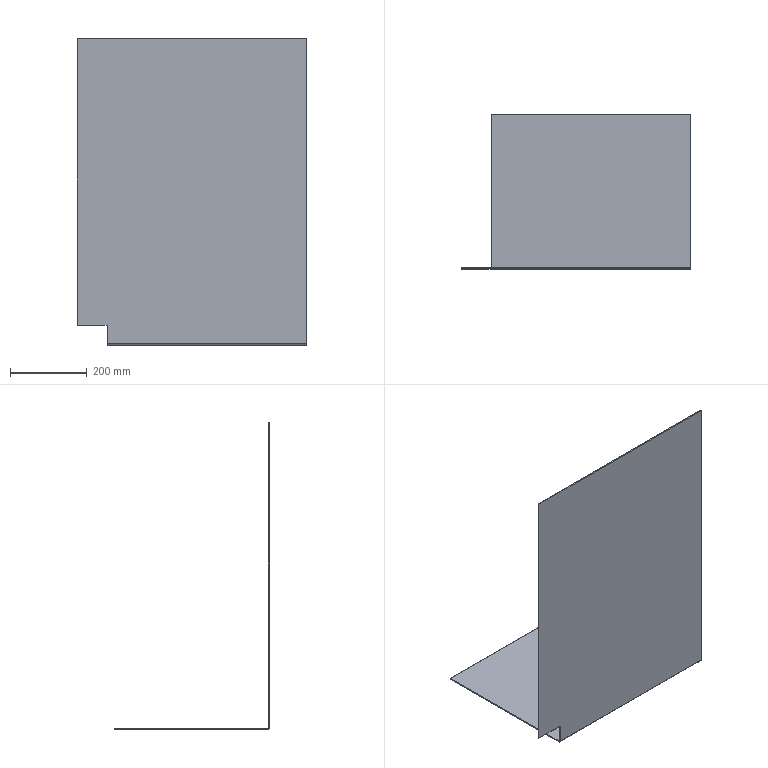Part | STEP file | E3-花纹Plate折弯5 | 1 solid | 14 faces | box 598 x 403 x 798 mm | volume 2041770 mm3 | plane 12 | cylinder 2 | commonest cylinder face diameters 2 x1 8 x1
STEP:
#1=CARTESIAN_POINT('',(0.,0.,0.));
#2=DIRECTION('',(0.,0.,1.));
#3=DIRECTION('',(1.,0.,0.));
#4=AXIS2_PLACEMENT_3D('',#1,#2,#3);
#5=CARTESIAN_POINT('',(598.,3.,-794.));
#6=VERTEX_POINT('',#5);
#7=CARTESIAN_POINT('',(598.,3.,0.));
#8=VERTEX_POINT('',#7);
#9=CARTESIAN_POINT('',(598.,3.,0.));
#10=DIRECTION('',(0.,0.,1.));
#11=VECTOR('',#10,1.);
#12=LINE('',#9,#11);
#13=CARTESIAN_POINT('',(598.,3.,0.));
#14=DIRECTION('',(1.,0.,0.));
#15=DIRECTION('',(0.,0.,1.));
#16=AXIS2_PLACEMENT_3D('',#13,#14,#15);
#17=PLANE('',#16);
#18=CARTESIAN_POINT('',(0.,0.));
#19=DIRECTION('',(1.,0.));
#20=VECTOR('',#19,1.);
#21=LINE('',#18,#20);
#22=(GEOMETRIC_REPRESENTATION_CONTEXT(2)PARAMETRIC_REPRESENTATION_CONTEXT()REPRESENTATION_CONTEXT('',''));
#23=DEFINITIONAL_REPRESENTATION('',(#21),#22);
#24=PCURVE('',#17,#23);
#25=CARTESIAN_POINT('',(0.,3.,0.));
#26=DIRECTION('',(0.,1.,0.));
#27=DIRECTION('',(0.,0.,-1.));
#28=AXIS2_PLACEMENT_3D('',#25,#26,#27);
#29=PLANE('',#28);
#30=CARTESIAN_POINT('',(0.,-598.));
#31=DIRECTION('',(-1.,0.));
#32=VECTOR('',#31,1.);
#33=LINE('',#30,#32);
#34=(GEOMETRIC_REPRESENTATION_CONTEXT(2)PARAMETRIC_REPRESENTATION_CONTEXT()REPRESENTATION_CONTEXT('',''));
#35=DEFINITIONAL_REPRESENTATION('',(#33),#34);
#36=PCURVE('',#29,#35);
#37=SURFACE_CURVE('',#12,(#24,#36),.PCURVE_S1.);
#38=EDGE_CURVE('',#6,#8,#37,.T.);
#39=ORIENTED_EDGE('',*,*,#38,.T.);
#40=CARTESIAN_POINT('',(598.,0.,0.));
#41=VERTEX_POINT('',#40);
#42=CARTESIAN_POINT('',(598.,3.,0.));
#43=DIRECTION('',(0.,1.,0.));
#44=VECTOR('',#43,1.);
#45=LINE('',#42,#44);
#46=CARTESIAN_POINT('',(0.,0.));
#47=DIRECTION('',(0.,-1.));
#48=VECTOR('',#47,1.);
#49=LINE('',#46,#48);
#50=(GEOMETRIC_REPRESENTATION_CONTEXT(2)PARAMETRIC_REPRESENTATION_CONTEXT()REPRESENTATION_CONTEXT('',''));
#51=DEFINITIONAL_REPRESENTATION('',(#49),#50);
#52=PCURVE('',#17,#51);
#53=CARTESIAN_POINT('',(0.,3.,0.));
#54=DIRECTION('',(0.,0.,1.));
#55=DIRECTION('',(-1.,0.,0.));
#56=AXIS2_PLACEMENT_3D('',#53,#54,#55);
#57=PLANE('',#56);
#58=CARTESIAN_POINT('',(-598.,0.));
#59=DIRECTION('',(0.,-1.));
#60=VECTOR('',#59,1.);
#61=LINE('',#58,#60);
#62=(GEOMETRIC_REPRESENTATION_CONTEXT(2)PARAMETRIC_REPRESENTATION_CONTEXT()REPRESENTATION_CONTEXT('',''));
#63=DEFINITIONAL_REPRESENTATION('',(#61),#62);
#64=PCURVE('',#57,#63);
#65=SURFACE_CURVE('',#45,(#52,#64),.PCURVE_S1.);
#66=EDGE_CURVE('',#41,#8,#65,.T.);
#67=ORIENTED_EDGE('',*,*,#66,.F.);
#68=CARTESIAN_POINT('',(598.,0.,-794.));
#69=VERTEX_POINT('',#68);
#70=CARTESIAN_POINT('',(598.,0.,0.));
#71=DIRECTION('',(0.,0.,1.));
#72=VECTOR('',#71,1.);
#73=LINE('',#70,#72);
#74=CARTESIAN_POINT('',(0.,3.));
#75=DIRECTION('',(1.,0.));
#76=VECTOR('',#75,1.);
#77=LINE('',#74,#76);
#78=(GEOMETRIC_REPRESENTATION_CONTEXT(2)PARAMETRIC_REPRESENTATION_CONTEXT()REPRESENTATION_CONTEXT('',''));
#79=DEFINITIONAL_REPRESENTATION('',(#77),#78);
#80=PCURVE('',#17,#79);
#81=CARTESIAN_POINT('',(0.,0.,0.));
#82=DIRECTION('',(0.,1.,0.));
#83=DIRECTION('',(0.,0.,-1.));
#84=AXIS2_PLACEMENT_3D('',#81,#82,#83);
#85=PLANE('',#84);
#86=CARTESIAN_POINT('',(0.,-598.));
#87=DIRECTION('',(-1.,0.));
#88=VECTOR('',#87,1.);
#89=LINE('',#86,#88);
#90=(GEOMETRIC_REPRESENTATION_CONTEXT(2)PARAMETRIC_REPRESENTATION_CONTEXT()REPRESENTATION_CONTEXT('',''));
#91=DEFINITIONAL_REPRESENTATION('',(#89),#90);
#92=PCURVE('',#85,#91);
#93=SURFACE_CURVE('',#73,(#80,#92),.PCURVE_S1.);
#94=EDGE_CURVE('',#69,#41,#93,.T.);
#95=ORIENTED_EDGE('',*,*,#94,.F.);
#96=CARTESIAN_POINT('',(598.,3.,-794.));
#97=DIRECTION('',(0.,-1.,0.));
#98=VECTOR('',#97,1.);
#99=LINE('',#96,#98);
#100=CARTESIAN_POINT('',(-794.,0.));
#101=DIRECTION('',(0.,1.));
#102=VECTOR('',#101,1.);
#103=LINE('',#100,#102);
#104=(GEOMETRIC_REPRESENTATION_CONTEXT(2)PARAMETRIC_REPRESENTATION_CONTEXT()REPRESENTATION_CONTEXT('',''));
#105=DEFINITIONAL_REPRESENTATION('',(#103),#104);
#106=PCURVE('',#17,#105);
#107=CARTESIAN_POINT('',(598.,4.,-794.));
#108=DIRECTION('',(-1.,0.,0.));
#109=DIRECTION('',(0.,0.,-1.));
#110=AXIS2_PLACEMENT_3D('',#107,#108,#109);
#111=PLANE('',#110);
#112=CARTESIAN_POINT('',(0.,1.));
#113=DIRECTION('',(0.,1.));
#114=VECTOR('',#113,1.);
#115=LINE('',#112,#114);
#116=(GEOMETRIC_REPRESENTATION_CONTEXT(2)PARAMETRIC_REPRESENTATION_CONTEXT()REPRESENTATION_CONTEXT('',''));
#117=DEFINITIONAL_REPRESENTATION('',(#115),#116);
#118=PCURVE('',#111,#117);
#119=SURFACE_CURVE('',#99,(#106,#118),.PCURVE_S1.);
#120=EDGE_CURVE('',#6,#69,#119,.T.);
#121=ORIENTED_EDGE('',*,*,#120,.F.);
#122=EDGE_LOOP('',(#39,#67,#95,#121));
#123=FACE_BOUND('',#122,.T.);
#124=ADVANCED_FACE('',(#123),#17,.T.);
#125=CARTESIAN_POINT('',(78.,3.,-746.));
#126=VERTEX_POINT('',#125);
#127=CARTESIAN_POINT('',(0.,3.,-746.));
#128=VERTEX_POINT('',#127);
#129=CARTESIAN_POINT('',(0.,3.,-746.));
#130=DIRECTION('',(-1.,0.,0.));
#131=VECTOR('',#130,1.);
#132=LINE('',#129,#131);
#133=CARTESIAN_POINT('',(746.,0.));
#134=DIRECTION('',(0.,1.));
#135=VECTOR('',#134,1.);
#136=LINE('',#133,#135);
#137=(GEOMETRIC_REPRESENTATION_CONTEXT(2)PARAMETRIC_REPRESENTATION_CONTEXT()REPRESENTATION_CONTEXT('',''));
#138=DEFINITIONAL_REPRESENTATION('',(#136),#137);
#139=PCURVE('',#29,#138);
#140=CARTESIAN_POINT('',(-82.,-497.,-746.));
#141=DIRECTION('',(0.,0.,1.));
#142=DIRECTION('',(-1.,0.,0.));
#143=AXIS2_PLACEMENT_3D('',#140,#141,#142);
#144=PLANE('',#143);
#145=CARTESIAN_POINT('',(-82.,-500.));
#146=DIRECTION('',(1.,0.));
#147=VECTOR('',#146,1.);
#148=LINE('',#145,#147);
#149=(GEOMETRIC_REPRESENTATION_CONTEXT(2)PARAMETRIC_REPRESENTATION_CONTEXT()REPRESENTATION_CONTEXT('',''));
#150=DEFINITIONAL_REPRESENTATION('',(#148),#149);
#151=PCURVE('',#144,#150);
#152=SURFACE_CURVE('',#132,(#139,#151),.PCURVE_S1.);
#153=EDGE_CURVE('',#126,#128,#152,.T.);
#154=ORIENTED_EDGE('',*,*,#153,.T.);
#155=CARTESIAN_POINT('',(0.,3.,0.));
#156=VERTEX_POINT('',#155);
#157=CARTESIAN_POINT('',(0.,3.,0.));
#158=DIRECTION('',(0.,0.,-1.));
#159=VECTOR('',#158,1.);
#160=LINE('',#157,#159);
#161=CARTESIAN_POINT('',(0.,0.));
#162=DIRECTION('',(1.,0.));
#163=VECTOR('',#162,1.);
#164=LINE('',#161,#163);
#165=(GEOMETRIC_REPRESENTATION_CONTEXT(2)PARAMETRIC_REPRESENTATION_CONTEXT()REPRESENTATION_CONTEXT('',''));
#166=DEFINITIONAL_REPRESENTATION('',(#164),#165);
#167=PCURVE('',#29,#166);
#168=CARTESIAN_POINT('',(0.,3.,0.));
#169=DIRECTION('',(-1.,0.,0.));
#170=DIRECTION('',(0.,0.,-1.));
#171=AXIS2_PLACEMENT_3D('',#168,#169,#170);
#172=PLANE('',#171);
#173=CARTESIAN_POINT('',(0.,0.));
#174=DIRECTION('',(1.,0.));
#175=VECTOR('',#174,1.);
#176=LINE('',#173,#175);
#177=(GEOMETRIC_REPRESENTATION_CONTEXT(2)PARAMETRIC_REPRESENTATION_CONTEXT()REPRESENTATION_CONTEXT('',''));
#178=DEFINITIONAL_REPRESENTATION('',(#176),#177);
#179=PCURVE('',#172,#178);
#180=SURFACE_CURVE('',#160,(#167,#179),.PCURVE_S1.);
#181=EDGE_CURVE('',#156,#128,#180,.T.);
#182=ORIENTED_EDGE('',*,*,#181,.F.);
#183=CARTESIAN_POINT('',(0.,3.,0.));
#184=DIRECTION('',(-1.,0.,0.));
#185=VECTOR('',#184,1.);
#186=LINE('',#183,#185);
#187=CARTESIAN_POINT('',(0.,0.));
#188=DIRECTION('',(0.,1.));
#189=VECTOR('',#188,1.);
#190=LINE('',#187,#189);
#191=(GEOMETRIC_REPRESENTATION_CONTEXT(2)PARAMETRIC_REPRESENTATION_CONTEXT()REPRESENTATION_CONTEXT('',''));
#192=DEFINITIONAL_REPRESENTATION('',(#190),#191);
#193=PCURVE('',#29,#192);
#194=CARTESIAN_POINT('',(0.,0.));
#195=DIRECTION('',(1.,0.));
#196=VECTOR('',#195,1.);
#197=LINE('',#194,#196);
#198=(GEOMETRIC_REPRESENTATION_CONTEXT(2)PARAMETRIC_REPRESENTATION_CONTEXT()REPRESENTATION_CONTEXT('',''));
#199=DEFINITIONAL_REPRESENTATION('',(#197),#198);
#200=PCURVE('',#57,#199);
#201=SURFACE_CURVE('',#186,(#193,#200),.PCURVE_S1.);
#202=EDGE_CURVE('',#8,#156,#201,.T.);
#203=ORIENTED_EDGE('',*,*,#202,.F.);
#204=ORIENTED_EDGE('',*,*,#38,.F.);
#205=CARTESIAN_POINT('',(78.,3.,-794.));
#206=VERTEX_POINT('',#205);
#207=CARTESIAN_POINT('',(598.,3.,-794.));
#208=DIRECTION('',(-1.,0.,0.));
#209=VECTOR('',#208,1.);
#210=LINE('',#207,#209);
#211=CARTESIAN_POINT('',(794.,-598.));
#212=DIRECTION('',(0.,1.));
#213=VECTOR('',#212,1.);
#214=LINE('',#211,#213);
#215=(GEOMETRIC_REPRESENTATION_CONTEXT(2)PARAMETRIC_REPRESENTATION_CONTEXT()REPRESENTATION_CONTEXT('',''));
#216=DEFINITIONAL_REPRESENTATION('',(#214),#215);
#217=PCURVE('',#29,#216);
#218=CARTESIAN_POINT('',(598.,4.,-794.));
#219=DIRECTION('',(1.,0.,0.));
#220=DIRECTION('',(0.,0.,-1.));
#221=AXIS2_PLACEMENT_3D('',#218,#219,#220);
#222=CYLINDRICAL_SURFACE('',#221,1.);
#223=CARTESIAN_POINT('',(4.712,0.));
#224=DIRECTION('',(0.,-1.));
#225=VECTOR('',#224,1.);
#226=LINE('',#223,#225);
#227=(GEOMETRIC_REPRESENTATION_CONTEXT(2)PARAMETRIC_REPRESENTATION_CONTEXT()REPRESENTATION_CONTEXT('',''));
#228=DEFINITIONAL_REPRESENTATION('',(#226),#227);
#229=PCURVE('',#222,#228);
#230=SURFACE_CURVE('',#210,(#217,#229),.PCURVE_S1.);
#231=EDGE_CURVE('',#6,#206,#230,.T.);
#232=ORIENTED_EDGE('',*,*,#231,.T.);
#233=CARTESIAN_POINT('',(78.,3.,0.));
#234=DIRECTION('',(0.,0.,1.));
#235=VECTOR('',#234,1.);
#236=LINE('',#233,#235);
#237=CARTESIAN_POINT('',(0.,-78.));
#238=DIRECTION('',(-1.,0.));
#239=VECTOR('',#238,1.);
#240=LINE('',#237,#239);
#241=(GEOMETRIC_REPRESENTATION_CONTEXT(2)PARAMETRIC_REPRESENTATION_CONTEXT()REPRESENTATION_CONTEXT('',''));
#242=DEFINITIONAL_REPRESENTATION('',(#240),#241);
#243=PCURVE('',#29,#242);
#244=CARTESIAN_POINT('',(78.,-497.,-798.));
#245=DIRECTION('',(1.,0.,0.));
#246=DIRECTION('',(0.,0.,1.));
#247=AXIS2_PLACEMENT_3D('',#244,#245,#246);
#248=PLANE('',#247);
#249=CARTESIAN_POINT('',(798.,-500.));
#250=DIRECTION('',(1.,0.));
#251=VECTOR('',#250,1.);
#252=LINE('',#249,#251);
#253=(GEOMETRIC_REPRESENTATION_CONTEXT(2)PARAMETRIC_REPRESENTATION_CONTEXT()REPRESENTATION_CONTEXT('',''));
#254=DEFINITIONAL_REPRESENTATION('',(#252),#253);
#255=PCURVE('',#248,#254);
#256=SURFACE_CURVE('',#236,(#243,#255),.PCURVE_S1.);
#257=EDGE_CURVE('',#206,#126,#256,.T.);
#258=ORIENTED_EDGE('',*,*,#257,.T.);
#259=EDGE_LOOP('',(#154,#182,#203,#204,#232,#258));
#260=FACE_BOUND('',#259,.T.);
#261=ADVANCED_FACE('',(#260),#29,.T.);
#262=CARTESIAN_POINT('',(78.,0.,-794.));
#263=VERTEX_POINT('',#262);
#264=CARTESIAN_POINT('',(78.,0.,-746.));
#265=VERTEX_POINT('',#264);
#266=CARTESIAN_POINT('',(78.,0.,0.));
#267=DIRECTION('',(0.,0.,1.));
#268=VECTOR('',#267,1.);
#269=LINE('',#266,#268);
#270=CARTESIAN_POINT('',(0.,-78.));
#271=DIRECTION('',(-1.,0.));
#272=VECTOR('',#271,1.);
#273=LINE('',#270,#272);
#274=(GEOMETRIC_REPRESENTATION_CONTEXT(2)PARAMETRIC_REPRESENTATION_CONTEXT()REPRESENTATION_CONTEXT('',''));
#275=DEFINITIONAL_REPRESENTATION('',(#273),#274);
#276=PCURVE('',#85,#275);
#277=CARTESIAN_POINT('',(798.,-497.));
#278=DIRECTION('',(1.,0.));
#279=VECTOR('',#278,1.);
#280=LINE('',#277,#279);
#281=(GEOMETRIC_REPRESENTATION_CONTEXT(2)PARAMETRIC_REPRESENTATION_CONTEXT()REPRESENTATION_CONTEXT('',''));
#282=DEFINITIONAL_REPRESENTATION('',(#280),#281);
#283=PCURVE('',#248,#282);
#284=SURFACE_CURVE('',#269,(#276,#283),.PCURVE_S1.);
#285=EDGE_CURVE('',#263,#265,#284,.T.);
#286=ORIENTED_EDGE('',*,*,#285,.F.);
#287=CARTESIAN_POINT('',(598.,0.,-794.));
#288=DIRECTION('',(-1.,0.,0.));
#289=VECTOR('',#288,1.);
#290=LINE('',#287,#289);
#291=CARTESIAN_POINT('',(794.,-598.));
#292=DIRECTION('',(0.,1.));
#293=VECTOR('',#292,1.);
#294=LINE('',#291,#293);
#295=(GEOMETRIC_REPRESENTATION_CONTEXT(2)PARAMETRIC_REPRESENTATION_CONTEXT()REPRESENTATION_CONTEXT('',''));
#296=DEFINITIONAL_REPRESENTATION('',(#294),#295);
#297=PCURVE('',#85,#296);
#298=CARTESIAN_POINT('',(598.,4.,-794.));
#299=DIRECTION('',(1.,0.,0.));
#300=DIRECTION('',(0.,0.,-1.));
#301=AXIS2_PLACEMENT_3D('',#298,#299,#300);
#302=CYLINDRICAL_SURFACE('',#301,4.);
#303=CARTESIAN_POINT('',(4.712,0.));
#304=DIRECTION('',(0.,-1.));
#305=VECTOR('',#304,1.);
#306=LINE('',#303,#305);
#307=(GEOMETRIC_REPRESENTATION_CONTEXT(2)PARAMETRIC_REPRESENTATION_CONTEXT()REPRESENTATION_CONTEXT('',''));
#308=DEFINITIONAL_REPRESENTATION('',(#306),#307);
#309=PCURVE('',#302,#308);
#310=SURFACE_CURVE('',#290,(#297,#309),.PCURVE_S1.);
#311=EDGE_CURVE('',#69,#263,#310,.T.);
#312=ORIENTED_EDGE('',*,*,#311,.F.);
#313=ORIENTED_EDGE('',*,*,#94,.T.);
#314=CARTESIAN_POINT('',(0.,0.,0.));
#315=VERTEX_POINT('',#314);
#316=CARTESIAN_POINT('',(0.,0.,0.));
#317=DIRECTION('',(-1.,0.,0.));
#318=VECTOR('',#317,1.);
#319=LINE('',#316,#318);
#320=CARTESIAN_POINT('',(0.,0.));
#321=DIRECTION('',(0.,1.));
#322=VECTOR('',#321,1.);
#323=LINE('',#320,#322);
#324=(GEOMETRIC_REPRESENTATION_CONTEXT(2)PARAMETRIC_REPRESENTATION_CONTEXT()REPRESENTATION_CONTEXT('',''));
#325=DEFINITIONAL_REPRESENTATION('',(#323),#324);
#326=PCURVE('',#85,#325);
#327=CARTESIAN_POINT('',(0.,3.));
#328=DIRECTION('',(1.,0.));
#329=VECTOR('',#328,1.);
#330=LINE('',#327,#329);
#331=(GEOMETRIC_REPRESENTATION_CONTEXT(2)PARAMETRIC_REPRESENTATION_CONTEXT()REPRESENTATION_CONTEXT('',''));
#332=DEFINITIONAL_REPRESENTATION('',(#330),#331);
#333=PCURVE('',#57,#332);
#334=SURFACE_CURVE('',#319,(#326,#333),.PCURVE_S1.);
#335=EDGE_CURVE('',#41,#315,#334,.T.);
#336=ORIENTED_EDGE('',*,*,#335,.T.);
#337=CARTESIAN_POINT('',(0.,0.,-746.));
#338=VERTEX_POINT('',#337);
#339=CARTESIAN_POINT('',(0.,0.,0.));
#340=DIRECTION('',(0.,0.,-1.));
#341=VECTOR('',#340,1.);
#342=LINE('',#339,#341);
#343=CARTESIAN_POINT('',(0.,0.));
#344=DIRECTION('',(1.,0.));
#345=VECTOR('',#344,1.);
#346=LINE('',#343,#345);
#347=(GEOMETRIC_REPRESENTATION_CONTEXT(2)PARAMETRIC_REPRESENTATION_CONTEXT()REPRESENTATION_CONTEXT('',''));
#348=DEFINITIONAL_REPRESENTATION('',(#346),#347);
#349=PCURVE('',#85,#348);
#350=CARTESIAN_POINT('',(0.,3.));
#351=DIRECTION('',(1.,0.));
#352=VECTOR('',#351,1.);
#353=LINE('',#350,#352);
#354=(GEOMETRIC_REPRESENTATION_CONTEXT(2)PARAMETRIC_REPRESENTATION_CONTEXT()REPRESENTATION_CONTEXT('',''));
#355=DEFINITIONAL_REPRESENTATION('',(#353),#354);
#356=PCURVE('',#172,#355);
#357=SURFACE_CURVE('',#342,(#349,#356),.PCURVE_S1.);
#358=EDGE_CURVE('',#315,#338,#357,.T.);
#359=ORIENTED_EDGE('',*,*,#358,.T.);
#360=CARTESIAN_POINT('',(0.,0.,-746.));
#361=DIRECTION('',(-1.,0.,0.));
#362=VECTOR('',#361,1.);
#363=LINE('',#360,#362);
#364=CARTESIAN_POINT('',(746.,0.));
#365=DIRECTION('',(0.,1.));
#366=VECTOR('',#365,1.);
#367=LINE('',#364,#366);
#368=(GEOMETRIC_REPRESENTATION_CONTEXT(2)PARAMETRIC_REPRESENTATION_CONTEXT()REPRESENTATION_CONTEXT('',''));
#369=DEFINITIONAL_REPRESENTATION('',(#367),#368);
#370=PCURVE('',#85,#369);
#371=CARTESIAN_POINT('',(-82.,-497.));
#372=DIRECTION('',(1.,0.));
#373=VECTOR('',#372,1.);
#374=LINE('',#371,#373);
#375=(GEOMETRIC_REPRESENTATION_CONTEXT(2)PARAMETRIC_REPRESENTATION_CONTEXT()REPRESENTATION_CONTEXT('',''));
#376=DEFINITIONAL_REPRESENTATION('',(#374),#375);
#377=PCURVE('',#144,#376);
#378=SURFACE_CURVE('',#363,(#370,#377),.PCURVE_S1.);
#379=EDGE_CURVE('',#265,#338,#378,.T.);
#380=ORIENTED_EDGE('',*,*,#379,.F.);
#381=EDGE_LOOP('',(#286,#312,#313,#336,#359,#380));
#382=FACE_BOUND('',#381,.T.);
#383=ADVANCED_FACE('',(#382),#85,.F.);
#384=ORIENTED_EDGE('',*,*,#66,.T.);
#385=ORIENTED_EDGE('',*,*,#202,.T.);
#386=CARTESIAN_POINT('',(0.,3.,0.));
#387=DIRECTION('',(0.,1.,0.));
#388=VECTOR('',#387,1.);
#389=LINE('',#386,#388);
#390=CARTESIAN_POINT('',(0.,0.));
#391=DIRECTION('',(0.,-1.));
#392=VECTOR('',#391,1.);
#393=LINE('',#390,#392);
#394=(GEOMETRIC_REPRESENTATION_CONTEXT(2)PARAMETRIC_REPRESENTATION_CONTEXT()REPRESENTATION_CONTEXT('',''));
#395=DEFINITIONAL_REPRESENTATION('',(#393),#394);
#396=PCURVE('',#57,#395);
#397=CARTESIAN_POINT('',(0.,0.));
#398=DIRECTION('',(0.,-1.));
#399=VECTOR('',#398,1.);
#400=LINE('',#397,#399);
#401=(GEOMETRIC_REPRESENTATION_CONTEXT(2)PARAMETRIC_REPRESENTATION_CONTEXT()REPRESENTATION_CONTEXT('',''));
#402=DEFINITIONAL_REPRESENTATION('',(#400),#401);
#403=PCURVE('',#172,#402);
#404=SURFACE_CURVE('',#389,(#396,#403),.PCURVE_S1.);
#405=EDGE_CURVE('',#315,#156,#404,.T.);
#406=ORIENTED_EDGE('',*,*,#405,.F.);
#407=ORIENTED_EDGE('',*,*,#335,.F.);
#408=EDGE_LOOP('',(#384,#385,#406,#407));
#409=FACE_BOUND('',#408,.T.);
#410=ADVANCED_FACE('',(#409),#57,.T.);
#411=CARTESIAN_POINT('',(0.,3.,-746.));
#412=DIRECTION('',(0.,-1.,0.));
#413=VECTOR('',#412,1.);
#414=LINE('',#411,#413);
#415=CARTESIAN_POINT('',(746.,0.));
#416=DIRECTION('',(0.,1.));
#417=VECTOR('',#416,1.);
#418=LINE('',#415,#417);
#419=(GEOMETRIC_REPRESENTATION_CONTEXT(2)PARAMETRIC_REPRESENTATION_CONTEXT()REPRESENTATION_CONTEXT('',''));
#420=DEFINITIONAL_REPRESENTATION('',(#418),#419);
#421=PCURVE('',#172,#420);
#422=CARTESIAN_POINT('',(-82.,-500.));
#423=DIRECTION('',(0.,1.));
#424=VECTOR('',#423,1.);
#425=LINE('',#422,#424);
#426=(GEOMETRIC_REPRESENTATION_CONTEXT(2)PARAMETRIC_REPRESENTATION_CONTEXT()REPRESENTATION_CONTEXT('',''));
#427=DEFINITIONAL_REPRESENTATION('',(#425),#426);
#428=PCURVE('',#144,#427);
#429=SURFACE_CURVE('',#414,(#421,#428),.PCURVE_S1.);
#430=EDGE_CURVE('',#128,#338,#429,.T.);
#431=ORIENTED_EDGE('',*,*,#430,.T.);
#432=ORIENTED_EDGE('',*,*,#358,.F.);
#433=ORIENTED_EDGE('',*,*,#405,.T.);
#434=ORIENTED_EDGE('',*,*,#181,.T.);
#435=EDGE_LOOP('',(#431,#432,#433,#434));
#436=FACE_BOUND('',#435,.T.);
#437=ADVANCED_FACE('',(#436),#172,.T.);
#438=CARTESIAN_POINT('',(598.,4.,-795.));
#439=VERTEX_POINT('',#438);
#440=CARTESIAN_POINT('',(598.,4.,-794.));
#441=DIRECTION('',(-1.,0.,0.));
#442=DIRECTION('',(0.,0.,1.));
#443=AXIS2_PLACEMENT_3D('',#440,#441,#442);
#444=CIRCLE('',#443,1.);
#445=CARTESIAN_POINT('',(0.,0.));
#446=DIRECTION('',(-1.,0.));
#447=AXIS2_PLACEMENT_2D('',#445,#446);
#448=CIRCLE('',#447,1.);
#449=(GEOMETRIC_REPRESENTATION_CONTEXT(2)PARAMETRIC_REPRESENTATION_CONTEXT()REPRESENTATION_CONTEXT('',''));
#450=DEFINITIONAL_REPRESENTATION('',(#448),#449);
#451=PCURVE('',#111,#450);
#452=CARTESIAN_POINT('',(9.425,0.));
#453=DIRECTION('',(-1.,0.));
#454=VECTOR('',#453,1.);
#455=LINE('',#452,#454);
#456=(GEOMETRIC_REPRESENTATION_CONTEXT(2)PARAMETRIC_REPRESENTATION_CONTEXT()REPRESENTATION_CONTEXT('',''));
#457=DEFINITIONAL_REPRESENTATION('',(#455),#456);
#458=PCURVE('',#222,#457);
#459=SURFACE_CURVE('',#444,(#451,#458),.PCURVE_S1.);
#460=EDGE_CURVE('',#439,#6,#459,.T.);
#461=ORIENTED_EDGE('',*,*,#460,.T.);
#462=ORIENTED_EDGE('',*,*,#120,.T.);
#463=CARTESIAN_POINT('',(598.,4.,-798.));
#464=VERTEX_POINT('',#463);
#465=CARTESIAN_POINT('',(598.,4.,-794.));
#466=DIRECTION('',(-1.,0.,0.));
#467=DIRECTION('',(0.,0.,1.));
#468=AXIS2_PLACEMENT_3D('',#465,#466,#467);
#469=CIRCLE('',#468,4.);
#470=CARTESIAN_POINT('',(0.,0.));
#471=DIRECTION('',(-1.,0.));
#472=AXIS2_PLACEMENT_2D('',#470,#471);
#473=CIRCLE('',#472,4.);
#474=(GEOMETRIC_REPRESENTATION_CONTEXT(2)PARAMETRIC_REPRESENTATION_CONTEXT()REPRESENTATION_CONTEXT('',''));
#475=DEFINITIONAL_REPRESENTATION('',(#473),#474);
#476=PCURVE('',#111,#475);
#477=CARTESIAN_POINT('',(9.425,0.));
#478=DIRECTION('',(-1.,0.));
#479=VECTOR('',#478,1.);
#480=LINE('',#477,#479);
#481=(GEOMETRIC_REPRESENTATION_CONTEXT(2)PARAMETRIC_REPRESENTATION_CONTEXT()REPRESENTATION_CONTEXT('',''));
#482=DEFINITIONAL_REPRESENTATION('',(#480),#481);
#483=PCURVE('',#302,#482);
#484=SURFACE_CURVE('',#469,(#476,#483),.PCURVE_S1.);
#485=EDGE_CURVE('',#464,#69,#484,.T.);
#486=ORIENTED_EDGE('',*,*,#485,.F.);
#487=CARTESIAN_POINT('',(598.,4.,-795.));
#488=DIRECTION('',(0.,0.,-1.));
#489=VECTOR('',#488,1.);
#490=LINE('',#487,#489);
#491=CARTESIAN_POINT('',(1.,0.));
#492=DIRECTION('',(1.,0.));
#493=VECTOR('',#492,1.);
#494=LINE('',#491,#493);
#495=(GEOMETRIC_REPRESENTATION_CONTEXT(2)PARAMETRIC_REPRESENTATION_CONTEXT()REPRESENTATION_CONTEXT('',''));
#496=DEFINITIONAL_REPRESENTATION('',(#494),#495);
#497=PCURVE('',#111,#496);
#498=CARTESIAN_POINT('',(598.,403.,-798.));
#499=DIRECTION('',(-1.,0.,0.));
#500=DIRECTION('',(0.,0.,-1.));
#501=AXIS2_PLACEMENT_3D('',#498,#499,#500);
#502=PLANE('',#501);
#503=CARTESIAN_POINT('',(-3.,399.));
#504=DIRECTION('',(1.,0.));
#505=VECTOR('',#504,1.);
#506=LINE('',#503,#505);
#507=(GEOMETRIC_REPRESENTATION_CONTEXT(2)PARAMETRIC_REPRESENTATION_CONTEXT()REPRESENTATION_CONTEXT('',''));
#508=DEFINITIONAL_REPRESENTATION('',(#506),#507);
#509=PCURVE('',#502,#508);
#510=SURFACE_CURVE('',#490,(#497,#509),.PCURVE_S1.);
#511=EDGE_CURVE('',#439,#464,#510,.T.);
#512=ORIENTED_EDGE('',*,*,#511,.F.);
#513=EDGE_LOOP('',(#461,#462,#486,#512));
#514=FACE_BOUND('',#513,.T.);
#515=ADVANCED_FACE('',(#514),#111,.F.);
#516=CARTESIAN_POINT('',(78.,4.,-798.));
#517=VERTEX_POINT('',#516);
#518=CARTESIAN_POINT('',(78.,4.,-794.));
#519=DIRECTION('',(1.,0.,0.));
#520=DIRECTION('',(0.,0.,1.));
#521=AXIS2_PLACEMENT_3D('',#518,#519,#520);
#522=CIRCLE('',#521,4.);
#523=CARTESIAN_POINT('',(3.142,-520.));
#524=DIRECTION('',(1.,0.));
#525=VECTOR('',#524,1.);
#526=LINE('',#523,#525);
#527=(GEOMETRIC_REPRESENTATION_CONTEXT(2)PARAMETRIC_REPRESENTATION_CONTEXT()REPRESENTATION_CONTEXT('',''));
#528=DEFINITIONAL_REPRESENTATION('',(#526),#527);
#529=PCURVE('',#302,#528);
#530=CARTESIAN_POINT('',(4.,-501.));
#531=DIRECTION('',(1.,0.));
#532=AXIS2_PLACEMENT_2D('',#530,#531);
#533=CIRCLE('',#532,4.);
#534=(GEOMETRIC_REPRESENTATION_CONTEXT(2)PARAMETRIC_REPRESENTATION_CONTEXT()REPRESENTATION_CONTEXT('',''));
#535=DEFINITIONAL_REPRESENTATION('',(#533),#534);
#536=PCURVE('',#248,#535);
#537=SURFACE_CURVE('',#522,(#529,#536),.PCURVE_S1.);
#538=EDGE_CURVE('',#263,#517,#537,.T.);
#539=ORIENTED_EDGE('',*,*,#538,.T.);
#540=CARTESIAN_POINT('',(0.,4.,-798.));
#541=DIRECTION('',(-1.,0.,0.));
#542=VECTOR('',#541,1.);
#543=LINE('',#540,#542);
#544=CARTESIAN_POINT('',(6.283,-598.));
#545=DIRECTION('',(0.,-1.));
#546=VECTOR('',#545,1.);
#547=LINE('',#544,#546);
#548=(GEOMETRIC_REPRESENTATION_CONTEXT(2)PARAMETRIC_REPRESENTATION_CONTEXT()REPRESENTATION_CONTEXT('',''));
#549=DEFINITIONAL_REPRESENTATION('',(#547),#548);
#550=PCURVE('',#302,#549);
#551=CARTESIAN_POINT('',(0.,0.,-798.));
#552=DIRECTION('',(0.,0.,1.));
#553=DIRECTION('',(-1.,0.,0.));
#554=AXIS2_PLACEMENT_3D('',#551,#552,#553);
#555=PLANE('',#554);
#556=CARTESIAN_POINT('',(0.,-4.));
#557=DIRECTION('',(1.,0.));
#558=VECTOR('',#557,1.);
#559=LINE('',#556,#558);
#560=(GEOMETRIC_REPRESENTATION_CONTEXT(2)PARAMETRIC_REPRESENTATION_CONTEXT()REPRESENTATION_CONTEXT('',''));
#561=DEFINITIONAL_REPRESENTATION('',(#559),#560);
#562=PCURVE('',#555,#561);
#563=SURFACE_CURVE('',#543,(#550,#562),.PCURVE_S1.);
#564=EDGE_CURVE('',#464,#517,#563,.T.);
#565=ORIENTED_EDGE('',*,*,#564,.F.);
#566=ORIENTED_EDGE('',*,*,#485,.T.);
#567=ORIENTED_EDGE('',*,*,#311,.T.);
#568=EDGE_LOOP('',(#539,#565,#566,#567));
#569=FACE_BOUND('',#568,.T.);
#570=ADVANCED_FACE('',(#569),#302,.T.);
#571=CARTESIAN_POINT('',(78.,4.,-795.));
#572=VERTEX_POINT('',#571);
#573=CARTESIAN_POINT('',(78.,4.,-794.));
#574=DIRECTION('',(1.,0.,0.));
#575=DIRECTION('',(0.,0.,1.));
#576=AXIS2_PLACEMENT_3D('',#573,#574,#575);
#577=CIRCLE('',#576,1.);
#578=CARTESIAN_POINT('',(3.142,-520.));
#579=DIRECTION('',(1.,0.));
#580=VECTOR('',#579,1.);
#581=LINE('',#578,#580);
#582=(GEOMETRIC_REPRESENTATION_CONTEXT(2)PARAMETRIC_REPRESENTATION_CONTEXT()REPRESENTATION_CONTEXT('',''));
#583=DEFINITIONAL_REPRESENTATION('',(#581),#582);
#584=PCURVE('',#222,#583);
#585=CARTESIAN_POINT('',(4.,-501.));
#586=DIRECTION('',(1.,0.));
#587=AXIS2_PLACEMENT_2D('',#585,#586);
#588=CIRCLE('',#587,1.);
#589=(GEOMETRIC_REPRESENTATION_CONTEXT(2)PARAMETRIC_REPRESENTATION_CONTEXT()REPRESENTATION_CONTEXT('',''));
#590=DEFINITIONAL_REPRESENTATION('',(#588),#589);
#591=PCURVE('',#248,#590);
#592=SURFACE_CURVE('',#577,(#584,#591),.PCURVE_S1.);
#593=EDGE_CURVE('',#206,#572,#592,.T.);
#594=ORIENTED_EDGE('',*,*,#593,.T.);
#595=CARTESIAN_POINT('',(0.,4.,-795.));
#596=DIRECTION('',(1.,0.,0.));
#597=VECTOR('',#596,1.);
#598=LINE('',#595,#597);
#599=CARTESIAN_POINT('',(6.283,-598.));
#600=DIRECTION('',(0.,1.));
#601=VECTOR('',#600,1.);
#602=LINE('',#599,#601);
#603=(GEOMETRIC_REPRESENTATION_CONTEXT(2)PARAMETRIC_REPRESENTATION_CONTEXT()REPRESENTATION_CONTEXT('',''));
#604=DEFINITIONAL_REPRESENTATION('',(#602),#603);
#605=PCURVE('',#222,#604);
#606=CARTESIAN_POINT('',(0.,0.,-795.));
#607=DIRECTION('',(0.,0.,1.));
#608=DIRECTION('',(-1.,0.,0.));
#609=AXIS2_PLACEMENT_3D('',#606,#607,#608);
#610=PLANE('',#609);
#611=CARTESIAN_POINT('',(0.,-4.));
#612=DIRECTION('',(-1.,0.));
#613=VECTOR('',#612,1.);
#614=LINE('',#611,#613);
#615=(GEOMETRIC_REPRESENTATION_CONTEXT(2)PARAMETRIC_REPRESENTATION_CONTEXT()REPRESENTATION_CONTEXT('',''));
#616=DEFINITIONAL_REPRESENTATION('',(#614),#615);
#617=PCURVE('',#610,#616);
#618=SURFACE_CURVE('',#598,(#605,#617),.PCURVE_S1.);
#619=EDGE_CURVE('',#572,#439,#618,.T.);
#620=ORIENTED_EDGE('',*,*,#619,.T.);
#621=ORIENTED_EDGE('',*,*,#460,.T.);
#622=ORIENTED_EDGE('',*,*,#231,.T.);
#623=EDGE_LOOP('',(#594,#620,#621,#622));
#624=FACE_BOUND('',#623,.F.);
#625=ADVANCED_FACE('',(#624),#222,.F.);
#626=ORIENTED_EDGE('',*,*,#511,.T.);
#627=CARTESIAN_POINT('',(598.,403.,-798.));
#628=VERTEX_POINT('',#627);
#629=CARTESIAN_POINT('',(598.,0.,-798.));
#630=DIRECTION('',(0.,1.,0.));
#631=VECTOR('',#630,1.);
#632=LINE('',#629,#631);
#633=CARTESIAN_POINT('',(0.,403.));
#634=DIRECTION('',(0.,-1.));
#635=VECTOR('',#634,1.);
#636=LINE('',#633,#635);
#637=(GEOMETRIC_REPRESENTATION_CONTEXT(2)PARAMETRIC_REPRESENTATION_CONTEXT()REPRESENTATION_CONTEXT('',''));
#638=DEFINITIONAL_REPRESENTATION('',(#636),#637);
#639=PCURVE('',#502,#638);
#640=CARTESIAN_POINT('',(-598.,0.));
#641=DIRECTION('',(0.,-1.));
#642=VECTOR('',#641,1.);
#643=LINE('',#640,#642);
#644=(GEOMETRIC_REPRESENTATION_CONTEXT(2)PARAMETRIC_REPRESENTATION_CONTEXT()REPRESENTATION_CONTEXT('',''));
#645=DEFINITIONAL_REPRESENTATION('',(#643),#644);
#646=PCURVE('',#555,#645);
#647=SURFACE_CURVE('',#632,(#639,#646),.PCURVE_S1.);
#648=EDGE_CURVE('',#464,#628,#647,.T.);
#649=ORIENTED_EDGE('',*,*,#648,.T.);
#650=CARTESIAN_POINT('',(598.,403.,-795.));
#651=VERTEX_POINT('',#650);
#652=CARTESIAN_POINT('',(598.,403.,-798.));
#653=DIRECTION('',(0.,0.,1.));
#654=VECTOR('',#653,1.);
#655=LINE('',#652,#654);
#656=CARTESIAN_POINT('',(0.,0.));
#657=DIRECTION('',(-1.,0.));
#658=VECTOR('',#657,1.);
#659=LINE('',#656,#658);
#660=(GEOMETRIC_REPRESENTATION_CONTEXT(2)PARAMETRIC_REPRESENTATION_CONTEXT()REPRESENTATION_CONTEXT('',''));
#661=DEFINITIONAL_REPRESENTATION('',(#659),#660);
#662=PCURVE('',#502,#661);
#663=CARTESIAN_POINT('',(0.,403.,-798.));
#664=DIRECTION('',(0.,-1.,0.));
#665=DIRECTION('',(0.,0.,1.));
#666=AXIS2_PLACEMENT_3D('',#663,#664,#665);
#667=PLANE('',#666);
#668=CARTESIAN_POINT('',(0.,-598.));
#669=DIRECTION('',(1.,0.));
#670=VECTOR('',#669,1.);
#671=LINE('',#668,#670);
#672=(GEOMETRIC_REPRESENTATION_CONTEXT(2)PARAMETRIC_REPRESENTATION_CONTEXT()REPRESENTATION_CONTEXT('',''));
#673=DEFINITIONAL_REPRESENTATION('',(#671),#672);
#674=PCURVE('',#667,#673);
#675=SURFACE_CURVE('',#655,(#662,#674),.PCURVE_S1.);
#676=EDGE_CURVE('',#628,#651,#675,.T.);
#677=ORIENTED_EDGE('',*,*,#676,.T.);
#678=CARTESIAN_POINT('',(598.,403.,-795.));
#679=DIRECTION('',(0.,1.,0.));
#680=VECTOR('',#679,1.);
#681=LINE('',#678,#680);
#682=CARTESIAN_POINT('',(-3.,0.));
#683=DIRECTION('',(0.,-1.));
#684=VECTOR('',#683,1.);
#685=LINE('',#682,#684);
#686=(GEOMETRIC_REPRESENTATION_CONTEXT(2)PARAMETRIC_REPRESENTATION_CONTEXT()REPRESENTATION_CONTEXT('',''));
#687=DEFINITIONAL_REPRESENTATION('',(#685),#686);
#688=PCURVE('',#502,#687);
#689=CARTESIAN_POINT('',(-598.,-403.));
#690=DIRECTION('',(0.,-1.));
#691=VECTOR('',#690,1.);
#692=LINE('',#689,#691);
#693=(GEOMETRIC_REPRESENTATION_CONTEXT(2)PARAMETRIC_REPRESENTATION_CONTEXT()REPRESENTATION_CONTEXT('',''));
#694=DEFINITIONAL_REPRESENTATION('',(#692),#693);
#695=PCURVE('',#610,#694);
#696=SURFACE_CURVE('',#681,(#688,#695),.PCURVE_S1.);
#697=EDGE_CURVE('',#439,#651,#696,.T.);
#698=ORIENTED_EDGE('',*,*,#697,.F.);
#699=EDGE_LOOP('',(#626,#649,#677,#698));
#700=FACE_BOUND('',#699,.T.);
#701=ADVANCED_FACE('',(#700),#502,.F.);
#702=CARTESIAN_POINT('',(78.,403.,-798.));
#703=VERTEX_POINT('',#702);
#704=CARTESIAN_POINT('',(0.,403.,-798.));
#705=DIRECTION('',(-1.,0.,0.));
#706=VECTOR('',#705,1.);
#707=LINE('',#704,#706);
#708=CARTESIAN_POINT('',(0.,-403.));
#709=DIRECTION('',(1.,0.));
#710=VECTOR('',#709,1.);
#711=LINE('',#708,#710);
#712=(GEOMETRIC_REPRESENTATION_CONTEXT(2)PARAMETRIC_REPRESENTATION_CONTEXT()REPRESENTATION_CONTEXT('',''));
#713=DEFINITIONAL_REPRESENTATION('',(#711),#712);
#714=PCURVE('',#555,#713);
#715=CARTESIAN_POINT('',(0.,0.));
#716=DIRECTION('',(0.,1.));
#717=VECTOR('',#716,1.);
#718=LINE('',#715,#717);
#719=(GEOMETRIC_REPRESENTATION_CONTEXT(2)PARAMETRIC_REPRESENTATION_CONTEXT()REPRESENTATION_CONTEXT('',''));
#720=DEFINITIONAL_REPRESENTATION('',(#718),#719);
#721=PCURVE('',#667,#720);
#722=SURFACE_CURVE('',#707,(#714,#721),.PCURVE_S1.);
#723=EDGE_CURVE('',#628,#703,#722,.T.);
#724=ORIENTED_EDGE('',*,*,#723,.F.);
#725=ORIENTED_EDGE('',*,*,#648,.F.);
#726=ORIENTED_EDGE('',*,*,#564,.T.);
#727=CARTESIAN_POINT('',(78.,-497.,-798.));
#728=DIRECTION('',(0.,1.,0.));
#729=VECTOR('',#728,1.);
#730=LINE('',#727,#729);
#731=CARTESIAN_POINT('',(-78.,497.));
#732=DIRECTION('',(0.,-1.));
#733=VECTOR('',#732,1.);
#734=LINE('',#731,#733);
#735=(GEOMETRIC_REPRESENTATION_CONTEXT(2)PARAMETRIC_REPRESENTATION_CONTEXT()REPRESENTATION_CONTEXT('',''));
#736=DEFINITIONAL_REPRESENTATION('',(#734),#735);
#737=PCURVE('',#555,#736);
#738=CARTESIAN_POINT('',(0.,0.));
#739=DIRECTION('',(0.,-1.));
#740=VECTOR('',#739,1.);
#741=LINE('',#738,#740);
#742=(GEOMETRIC_REPRESENTATION_CONTEXT(2)PARAMETRIC_REPRESENTATION_CONTEXT()REPRESENTATION_CONTEXT('',''));
#743=DEFINITIONAL_REPRESENTATION('',(#741),#742);
#744=PCURVE('',#248,#743);
#745=SURFACE_CURVE('',#730,(#737,#744),.PCURVE_S1.);
#746=EDGE_CURVE('',#517,#703,#745,.T.);
#747=ORIENTED_EDGE('',*,*,#746,.T.);
#748=EDGE_LOOP('',(#724,#725,#726,#747));
#749=FACE_BOUND('',#748,.T.);
#750=ADVANCED_FACE('',(#749),#555,.F.);
#751=CARTESIAN_POINT('',(78.,403.,-795.));
#752=VERTEX_POINT('',#751);
#753=CARTESIAN_POINT('',(78.,0.,-795.));
#754=DIRECTION('',(0.,-1.,0.));
#755=VECTOR('',#754,1.);
#756=LINE('',#753,#755);
#757=CARTESIAN_POINT('',(-78.,0.));
#758=DIRECTION('',(0.,1.));
#759=VECTOR('',#758,1.);
#760=LINE('',#757,#759);
#761=(GEOMETRIC_REPRESENTATION_CONTEXT(2)PARAMETRIC_REPRESENTATION_CONTEXT()REPRESENTATION_CONTEXT('',''));
#762=DEFINITIONAL_REPRESENTATION('',(#760),#761);
#763=PCURVE('',#610,#762);
#764=CARTESIAN_POINT('',(3.,-497.));
#765=DIRECTION('',(0.,1.));
#766=VECTOR('',#765,1.);
#767=LINE('',#764,#766);
#768=(GEOMETRIC_REPRESENTATION_CONTEXT(2)PARAMETRIC_REPRESENTATION_CONTEXT()REPRESENTATION_CONTEXT('',''));
#769=DEFINITIONAL_REPRESENTATION('',(#767),#768);
#770=PCURVE('',#248,#769);
#771=SURFACE_CURVE('',#756,(#763,#770),.PCURVE_S1.);
#772=EDGE_CURVE('',#752,#572,#771,.T.);
#773=ORIENTED_EDGE('',*,*,#772,.T.);
#774=ORIENTED_EDGE('',*,*,#619,.T.);
#775=ORIENTED_EDGE('',*,*,#697,.T.);
#776=CARTESIAN_POINT('',(0.,403.,-795.));
#777=DIRECTION('',(-1.,0.,0.));
#778=VECTOR('',#777,1.);
#779=LINE('',#776,#778);
#780=CARTESIAN_POINT('',(0.,-403.));
#781=DIRECTION('',(1.,0.));
#782=VECTOR('',#781,1.);
#783=LINE('',#780,#782);
#784=(GEOMETRIC_REPRESENTATION_CONTEXT(2)PARAMETRIC_REPRESENTATION_CONTEXT()REPRESENTATION_CONTEXT('',''));
#785=DEFINITIONAL_REPRESENTATION('',(#783),#784);
#786=PCURVE('',#610,#785);
#787=CARTESIAN_POINT('',(3.,0.));
#788=DIRECTION('',(0.,1.));
#789=VECTOR('',#788,1.);
#790=LINE('',#787,#789);
#791=(GEOMETRIC_REPRESENTATION_CONTEXT(2)PARAMETRIC_REPRESENTATION_CONTEXT()REPRESENTATION_CONTEXT('',''));
#792=DEFINITIONAL_REPRESENTATION('',(#790),#791);
#793=PCURVE('',#667,#792);
#794=SURFACE_CURVE('',#779,(#786,#793),.PCURVE_S1.);
#795=EDGE_CURVE('',#651,#752,#794,.T.);
#796=ORIENTED_EDGE('',*,*,#795,.T.);
#797=EDGE_LOOP('',(#773,#774,#775,#796));
#798=FACE_BOUND('',#797,.T.);
#799=ADVANCED_FACE('',(#798),#610,.T.);
#800=ORIENTED_EDGE('',*,*,#795,.F.);
#801=ORIENTED_EDGE('',*,*,#676,.F.);
#802=ORIENTED_EDGE('',*,*,#723,.T.);
#803=CARTESIAN_POINT('',(78.,403.,-798.));
#804=DIRECTION('',(0.,0.,-1.));
#805=VECTOR('',#804,1.);
#806=LINE('',#803,#805);
#807=CARTESIAN_POINT('',(0.,-78.));
#808=DIRECTION('',(-1.,0.));
#809=VECTOR('',#808,1.);
#810=LINE('',#807,#809);
#811=(GEOMETRIC_REPRESENTATION_CONTEXT(2)PARAMETRIC_REPRESENTATION_CONTEXT()REPRESENTATION_CONTEXT('',''));
#812=DEFINITIONAL_REPRESENTATION('',(#810),#811);
#813=PCURVE('',#667,#812);
#814=CARTESIAN_POINT('',(0.,-900.));
#815=DIRECTION('',(-1.,0.));
#816=VECTOR('',#815,1.);
#817=LINE('',#814,#816);
#818=(GEOMETRIC_REPRESENTATION_CONTEXT(2)PARAMETRIC_REPRESENTATION_CONTEXT()REPRESENTATION_CONTEXT('',''));
#819=DEFINITIONAL_REPRESENTATION('',(#817),#818);
#820=PCURVE('',#248,#819);
#821=SURFACE_CURVE('',#806,(#813,#820),.PCURVE_S1.);
#822=EDGE_CURVE('',#752,#703,#821,.T.);
#823=ORIENTED_EDGE('',*,*,#822,.F.);
#824=EDGE_LOOP('',(#800,#801,#802,#823));
#825=FACE_BOUND('',#824,.T.);
#826=ADVANCED_FACE('',(#825),#667,.F.);
#827=ORIENTED_EDGE('',*,*,#538,.F.);
#828=ORIENTED_EDGE('',*,*,#285,.T.);
#829=CARTESIAN_POINT('',(78.,-497.,-746.));
#830=DIRECTION('',(0.,1.,0.));
#831=VECTOR('',#830,1.);
#832=LINE('',#829,#831);
#833=CARTESIAN_POINT('',(52.,0.));
#834=DIRECTION('',(0.,-1.));
#835=VECTOR('',#834,1.);
#836=LINE('',#833,#835);
#837=(GEOMETRIC_REPRESENTATION_CONTEXT(2)PARAMETRIC_REPRESENTATION_CONTEXT()REPRESENTATION_CONTEXT('',''));
#838=DEFINITIONAL_REPRESENTATION('',(#836),#837);
#839=PCURVE('',#248,#838);
#840=CARTESIAN_POINT('',(-160.,0.));
#841=DIRECTION('',(0.,-1.));
#842=VECTOR('',#841,1.);
#843=LINE('',#840,#842);
#844=(GEOMETRIC_REPRESENTATION_CONTEXT(2)PARAMETRIC_REPRESENTATION_CONTEXT()REPRESENTATION_CONTEXT('',''));
#845=DEFINITIONAL_REPRESENTATION('',(#843),#844);
#846=PCURVE('',#144,#845);
#847=SURFACE_CURVE('',#832,(#839,#846),.PCURVE_S1.);
#848=EDGE_CURVE('',#265,#126,#847,.T.);
#849=ORIENTED_EDGE('',*,*,#848,.T.);
#850=ORIENTED_EDGE('',*,*,#257,.F.);
#851=ORIENTED_EDGE('',*,*,#593,.T.);
#852=ORIENTED_EDGE('',*,*,#772,.F.);
#853=ORIENTED_EDGE('',*,*,#822,.T.);
#854=ORIENTED_EDGE('',*,*,#746,.F.);
#855=EDGE_LOOP('',(#827,#828,#849,#850,#851,#852,#853,#854));
#856=FACE_BOUND('',#855,.T.);
#857=ADVANCED_FACE('',(#856),#248,.F.);
#858=ORIENTED_EDGE('',*,*,#153,.F.);
#859=ORIENTED_EDGE('',*,*,#848,.F.);
#860=ORIENTED_EDGE('',*,*,#379,.T.);
#861=ORIENTED_EDGE('',*,*,#430,.F.);
#862=EDGE_LOOP('',(#858,#859,#860,#861));
#863=FACE_BOUND('',#862,.T.);
#864=ADVANCED_FACE('',(#863),#144,.F.);
#865=CLOSED_SHELL('',(#124,#261,#383,#410,#437,#515,#570,#625,#701,#750,#799,#826,#857,#864));
#866=MANIFOLD_SOLID_BREP('',#865);
#867=(LENGTH_UNIT()NAMED_UNIT(*)SI_UNIT(.MILLI.,.METRE.));
#868=UNCERTAINTY_MEASURE_WITH_UNIT(LENGTH_MEASURE(0.0000001),#867,'','');
#869=(NAMED_UNIT(*)PLANE_ANGLE_UNIT()SI_UNIT($,.RADIAN.));
#870=(NAMED_UNIT(*)SI_UNIT($,.STERADIAN.)SOLID_ANGLE_UNIT());
#871=(GEOMETRIC_REPRESENTATION_CONTEXT(3)GLOBAL_UNCERTAINTY_ASSIGNED_CONTEXT((#868))GLOBAL_UNIT_ASSIGNED_CONTEXT((#867,#869,#870))REPRESENTATION_CONTEXT('',''));
#872=ADVANCED_BREP_SHAPE_REPRESENTATION('',(#4,#866),#871);